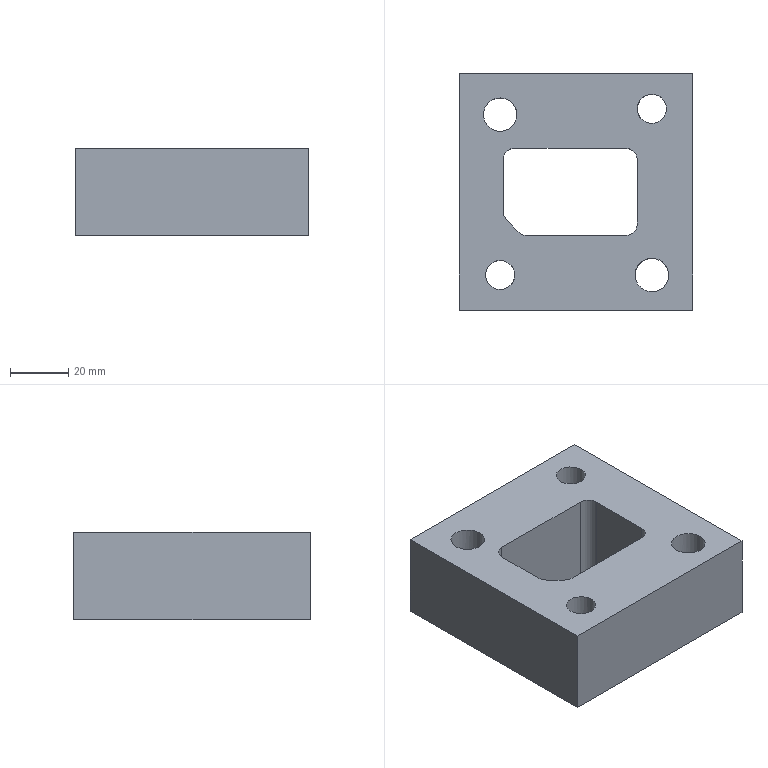Part | NX | features 7 2 | 1 solid | 28 faces | box 80 x 81 x 30 mm | volume 139031 mm3 | plane 15 | cylinder 13 | commonest cylinder face diameters 8 x5 10.001 x2 10.31 x2 11.5 x2 18 x2
STEP:
#1=CARTESIAN_POINT('',(3363.438,56.938,91.));
#2=VERTEX_POINT('',#1);
#3=CARTESIAN_POINT('',(3401.438,56.938,91.));
#4=VERTEX_POINT('',#3);
#5=CARTESIAN_POINT('',(3374.438,56.938,91.));
#6=DIRECTION('',(1.,0.,0.));
#7=VECTOR('',#6,1000.);
#8=LINE('',#5,#7);
#9=EDGE_CURVE('',#2,#4,#8,.T.);
#10=ORIENTED_EDGE('',*,*,#9,.T.);
#11=CARTESIAN_POINT('',(3405.438,52.938,91.));
#12=VERTEX_POINT('',#11);
#13=CARTESIAN_POINT('',(3401.438,52.938,91.));
#14=DIRECTION('',(0.,0.,1.));
#15=DIRECTION('',(0.,1.,0.));
#16=AXIS2_PLACEMENT_3D('',#13,#14,#15);
#17=CIRCLE('',#16,4.);
#18=EDGE_CURVE('',#12,#4,#17,.T.);
#19=ORIENTED_EDGE('',*,*,#18,.F.);
#20=CARTESIAN_POINT('',(3405.438,30.938,91.));
#21=VERTEX_POINT('',#20);
#22=CARTESIAN_POINT('',(3405.438,41.938,91.));
#23=DIRECTION('',(0.,-1.,0.));
#24=VECTOR('',#23,1000.);
#25=LINE('',#22,#24);
#26=EDGE_CURVE('',#12,#21,#25,.T.);
#27=ORIENTED_EDGE('',*,*,#26,.T.);
#28=CARTESIAN_POINT('',(3401.438,26.938,91.));
#29=VERTEX_POINT('',#28);
#30=CARTESIAN_POINT('',(3401.438,30.938,91.));
#31=DIRECTION('',(0.,0.,1.));
#32=DIRECTION('',(0.,1.,0.));
#33=AXIS2_PLACEMENT_3D('',#30,#31,#32);
#34=CIRCLE('',#33,4.);
#35=EDGE_CURVE('',#29,#21,#34,.T.);
#36=ORIENTED_EDGE('',*,*,#35,.F.);
#37=CARTESIAN_POINT('',(3367.731,26.938,91.));
#38=VERTEX_POINT('',#37);
#39=CARTESIAN_POINT('',(3374.438,26.938,91.));
#40=DIRECTION('',(-1.,0.,0.));
#41=VECTOR('',#40,1000.);
#42=LINE('',#39,#41);
#43=EDGE_CURVE('',#29,#38,#42,.T.);
#44=ORIENTED_EDGE('',*,*,#43,.T.);
#45=CARTESIAN_POINT('',(3364.902,28.11,91.));
#46=VERTEX_POINT('',#45);
#47=CARTESIAN_POINT('',(3367.731,30.938,91.));
#48=DIRECTION('',(0.,0.,1.));
#49=DIRECTION('',(0.,-1.,0.));
#50=AXIS2_PLACEMENT_3D('',#47,#48,#49);
#51=CIRCLE('',#50,4.);
#52=EDGE_CURVE('',#46,#38,#51,.T.);
#53=ORIENTED_EDGE('',*,*,#52,.F.);
#54=CARTESIAN_POINT('',(3360.609,32.403,91.));
#55=VERTEX_POINT('',#54);
#56=CARTESIAN_POINT('',(3364.006,29.006,91.));
#57=DIRECTION('',(0.7071,-0.7071,0.));
#58=VECTOR('',#57,1000.);
#59=LINE('',#56,#58);
#60=EDGE_CURVE('',#55,#46,#59,.T.);
#61=ORIENTED_EDGE('',*,*,#60,.F.);
#62=CARTESIAN_POINT('',(3359.438,35.231,91.));
#63=VERTEX_POINT('',#62);
#64=CARTESIAN_POINT('',(3363.438,35.231,91.));
#65=DIRECTION('',(0.,0.,1.));
#66=DIRECTION('',(0.,-1.,0.));
#67=AXIS2_PLACEMENT_3D('',#64,#65,#66);
#68=CIRCLE('',#67,4.);
#69=EDGE_CURVE('',#63,#55,#68,.T.);
#70=ORIENTED_EDGE('',*,*,#69,.F.);
#71=CARTESIAN_POINT('',(3359.438,52.938,91.));
#72=VERTEX_POINT('',#71);
#73=CARTESIAN_POINT('',(3359.438,41.938,91.));
#74=DIRECTION('',(0.,1.,0.));
#75=VECTOR('',#74,1000.);
#76=LINE('',#73,#75);
#77=EDGE_CURVE('',#63,#72,#76,.T.);
#78=ORIENTED_EDGE('',*,*,#77,.T.);
#79=CARTESIAN_POINT('',(3363.438,52.938,91.));
#80=DIRECTION('',(0.,0.,1.));
#81=DIRECTION('',(0.,-1.,0.));
#82=AXIS2_PLACEMENT_3D('',#79,#80,#81);
#83=CIRCLE('',#82,4.);
#84=EDGE_CURVE('',#2,#72,#83,.T.);
#85=ORIENTED_EDGE('',*,*,#84,.F.);
#86=EDGE_LOOP('',(#10,#19,#27,#36,#44,#53,#61,#70,#78,#85));
#87=FACE_BOUND('',#86,.T.);
#88=CARTESIAN_POINT('',(3410.438,75.439,91.));
#89=VERTEX_POINT('',#88);
#90=CARTESIAN_POINT('',(3410.438,70.438,91.));
#91=DIRECTION('',(0.,0.,-1.));
#92=DIRECTION('',(0.,1.,0.));
#93=AXIS2_PLACEMENT_3D('',#90,#91,#92);
#94=CIRCLE('',#93,5.);
#95=EDGE_CURVE('',#89,#89,#94,.T.);
#96=ORIENTED_EDGE('',*,*,#95,.T.);
#97=EDGE_LOOP('',(#96));
#98=FACE_BOUND('',#97,.T.);
#99=CARTESIAN_POINT('',(3358.438,74.188,91.));
#100=VERTEX_POINT('',#99);
#101=CARTESIAN_POINT('',(3358.438,68.438,91.));
#102=DIRECTION('',(0.,0.,1.));
#103=DIRECTION('',(0.,1.,0.));
#104=AXIS2_PLACEMENT_3D('',#101,#102,#103);
#105=CIRCLE('',#104,5.75);
#106=EDGE_CURVE('',#100,#100,#105,.T.);
#107=ORIENTED_EDGE('',*,*,#106,.F.);
#108=EDGE_LOOP('',(#107));
#109=FACE_BOUND('',#108,.T.);
#110=CARTESIAN_POINT('',(3424.438,1.438,91.));
#111=VERTEX_POINT('',#110);
#112=CARTESIAN_POINT('',(3344.438,1.438,91.));
#113=VERTEX_POINT('',#112);
#114=CARTESIAN_POINT('',(3374.438,1.438,91.));
#115=DIRECTION('',(-1.,0.,0.));
#116=VECTOR('',#115,1000.);
#117=LINE('',#114,#116);
#118=EDGE_CURVE('',#111,#113,#117,.T.);
#119=ORIENTED_EDGE('',*,*,#118,.F.);
#120=CARTESIAN_POINT('',(3424.438,82.438,91.));
#121=VERTEX_POINT('',#120);
#122=CARTESIAN_POINT('',(3424.438,41.938,91.));
#123=DIRECTION('',(0.,-1.,0.));
#124=VECTOR('',#123,1000.);
#125=LINE('',#122,#124);
#126=EDGE_CURVE('',#121,#111,#125,.T.);
#127=ORIENTED_EDGE('',*,*,#126,.F.);
#128=CARTESIAN_POINT('',(3344.438,82.438,91.));
#129=VERTEX_POINT('',#128);
#130=CARTESIAN_POINT('',(3374.438,82.438,91.));
#131=DIRECTION('',(1.,0.,0.));
#132=VECTOR('',#131,1000.);
#133=LINE('',#130,#132);
#134=EDGE_CURVE('',#129,#121,#133,.T.);
#135=ORIENTED_EDGE('',*,*,#134,.F.);
#136=CARTESIAN_POINT('',(3344.438,41.938,91.));
#137=DIRECTION('',(0.,1.,0.));
#138=VECTOR('',#137,1000.);
#139=LINE('',#136,#138);
#140=EDGE_CURVE('',#113,#129,#139,.T.);
#141=ORIENTED_EDGE('',*,*,#140,.F.);
#142=EDGE_LOOP('',(#119,#127,#135,#141));
#143=FACE_BOUND('',#142,.T.);
#144=CARTESIAN_POINT('',(3410.438,19.188,91.));
#145=VERTEX_POINT('',#144);
#146=CARTESIAN_POINT('',(3410.438,13.438,91.));
#147=DIRECTION('',(0.,0.,1.));
#148=DIRECTION('',(0.,1.,0.));
#149=AXIS2_PLACEMENT_3D('',#146,#147,#148);
#150=CIRCLE('',#149,5.75);
#151=EDGE_CURVE('',#145,#145,#150,.T.);
#152=ORIENTED_EDGE('',*,*,#151,.F.);
#153=EDGE_LOOP('',(#152));
#154=FACE_BOUND('',#153,.T.);
#155=CARTESIAN_POINT('',(3358.438,18.439,91.));
#156=VERTEX_POINT('',#155);
#157=CARTESIAN_POINT('',(3358.438,13.438,91.));
#158=DIRECTION('',(0.,0.,-1.));
#159=DIRECTION('',(0.,1.,0.));
#160=AXIS2_PLACEMENT_3D('',#157,#158,#159);
#161=CIRCLE('',#160,5.);
#162=EDGE_CURVE('',#156,#156,#161,.T.);
#163=ORIENTED_EDGE('',*,*,#162,.T.);
#164=EDGE_LOOP('',(#163));
#165=FACE_BOUND('',#164,.T.);
#166=CARTESIAN_POINT('',(3374.438,41.938,91.));
#167=DIRECTION('',(0.,0.,1.));
#168=DIRECTION('',(0.,-1.,0.));
#169=AXIS2_PLACEMENT_3D('',#166,#167,#168);
#170=PLANE('',#169);
#171=ADVANCED_FACE('',(#87,#98,#109,#143,#154,#165),#170,.T.);
#172=CARTESIAN_POINT('',(3415.593,70.438,61.));
#173=VERTEX_POINT('',#172);
#174=CARTESIAN_POINT('',(3410.438,70.438,61.));
#175=DIRECTION('',(0.,0.,1.));
#176=DIRECTION('',(1.,0.,0.));
#177=AXIS2_PLACEMENT_3D('',#174,#175,#176);
#178=CIRCLE('',#177,5.155);
#179=EDGE_CURVE('',#173,#173,#178,.T.);
#180=ORIENTED_EDGE('',*,*,#179,.T.);
#181=EDGE_LOOP('',(#180));
#182=FACE_BOUND('',#181,.T.);
#183=CARTESIAN_POINT('',(3363.593,13.438,61.));
#184=VERTEX_POINT('',#183);
#185=CARTESIAN_POINT('',(3358.438,13.438,61.));
#186=DIRECTION('',(0.,0.,1.));
#187=DIRECTION('',(1.,0.,0.));
#188=AXIS2_PLACEMENT_3D('',#185,#186,#187);
#189=CIRCLE('',#188,5.155);
#190=EDGE_CURVE('',#184,#184,#189,.T.);
#191=ORIENTED_EDGE('',*,*,#190,.T.);
#192=EDGE_LOOP('',(#191));
#193=FACE_BOUND('',#192,.T.);
#194=CARTESIAN_POINT('',(3359.438,52.938,61.));
#195=VERTEX_POINT('',#194);
#196=CARTESIAN_POINT('',(3363.438,56.938,61.));
#197=VERTEX_POINT('',#196);
#198=CARTESIAN_POINT('',(3363.438,52.938,61.));
#199=DIRECTION('',(0.,0.,-1.));
#200=DIRECTION('',(-1.,0.,0.));
#201=AXIS2_PLACEMENT_3D('',#198,#199,#200);
#202=CIRCLE('',#201,4.);
#203=EDGE_CURVE('',#195,#197,#202,.T.);
#204=ORIENTED_EDGE('',*,*,#203,.F.);
#205=CARTESIAN_POINT('',(3359.438,35.231,61.));
#206=VERTEX_POINT('',#205);
#207=CARTESIAN_POINT('',(3359.438,-135.062,61.));
#208=DIRECTION('',(0.,-1.,0.));
#209=VECTOR('',#208,1000.);
#210=LINE('',#207,#209);
#211=EDGE_CURVE('',#195,#206,#210,.T.);
#212=ORIENTED_EDGE('',*,*,#211,.T.);
#213=CARTESIAN_POINT('',(3360.609,32.403,61.));
#214=VERTEX_POINT('',#213);
#215=CARTESIAN_POINT('',(3363.438,35.231,61.));
#216=DIRECTION('',(0.,0.,-1.));
#217=DIRECTION('',(-1.,0.,0.));
#218=AXIS2_PLACEMENT_3D('',#215,#216,#217);
#219=CIRCLE('',#218,4.);
#220=EDGE_CURVE('',#214,#206,#219,.T.);
#221=ORIENTED_EDGE('',*,*,#220,.F.);
#222=CARTESIAN_POINT('',(3364.902,28.11,61.));
#223=VERTEX_POINT('',#222);
#224=CARTESIAN_POINT('',(3449.756,-56.744,61.));
#225=DIRECTION('',(-0.7071,0.7071,0.));
#226=VECTOR('',#225,1000.);
#227=LINE('',#224,#226);
#228=EDGE_CURVE('',#223,#214,#227,.T.);
#229=ORIENTED_EDGE('',*,*,#228,.F.);
#230=CARTESIAN_POINT('',(3367.731,26.938,61.));
#231=VERTEX_POINT('',#230);
#232=CARTESIAN_POINT('',(3367.731,30.938,61.));
#233=DIRECTION('',(0.,0.,-1.));
#234=DIRECTION('',(-1.,0.,0.));
#235=AXIS2_PLACEMENT_3D('',#232,#233,#234);
#236=CIRCLE('',#235,4.);
#237=EDGE_CURVE('',#231,#223,#236,.T.);
#238=ORIENTED_EDGE('',*,*,#237,.F.);
#239=CARTESIAN_POINT('',(3401.438,26.938,61.));
#240=VERTEX_POINT('',#239);
#241=CARTESIAN_POINT('',(3371.438,26.938,61.));
#242=DIRECTION('',(1.,0.,0.));
#243=VECTOR('',#242,1000.);
#244=LINE('',#241,#243);
#245=EDGE_CURVE('',#231,#240,#244,.T.);
#246=ORIENTED_EDGE('',*,*,#245,.T.);
#247=CARTESIAN_POINT('',(3405.438,30.938,61.));
#248=VERTEX_POINT('',#247);
#249=CARTESIAN_POINT('',(3401.438,30.938,61.));
#250=DIRECTION('',(0.,0.,-1.));
#251=DIRECTION('',(-1.,0.,0.));
#252=AXIS2_PLACEMENT_3D('',#249,#250,#251);
#253=CIRCLE('',#252,4.);
#254=EDGE_CURVE('',#248,#240,#253,.T.);
#255=ORIENTED_EDGE('',*,*,#254,.F.);
#256=CARTESIAN_POINT('',(3405.438,52.938,61.));
#257=VERTEX_POINT('',#256);
#258=CARTESIAN_POINT('',(3405.438,-135.062,61.));
#259=DIRECTION('',(0.,1.,0.));
#260=VECTOR('',#259,1000.);
#261=LINE('',#258,#260);
#262=EDGE_CURVE('',#248,#257,#261,.T.);
#263=ORIENTED_EDGE('',*,*,#262,.T.);
#264=CARTESIAN_POINT('',(3401.438,56.938,61.));
#265=VERTEX_POINT('',#264);
#266=CARTESIAN_POINT('',(3401.438,52.938,61.));
#267=DIRECTION('',(0.,0.,-1.));
#268=DIRECTION('',(-1.,0.,0.));
#269=AXIS2_PLACEMENT_3D('',#266,#267,#268);
#270=CIRCLE('',#269,4.);
#271=EDGE_CURVE('',#265,#257,#270,.T.);
#272=ORIENTED_EDGE('',*,*,#271,.F.);
#273=CARTESIAN_POINT('',(3371.438,56.938,61.));
#274=DIRECTION('',(-1.,0.,0.));
#275=VECTOR('',#274,1000.);
#276=LINE('',#273,#275);
#277=EDGE_CURVE('',#265,#197,#276,.T.);
#278=ORIENTED_EDGE('',*,*,#277,.T.);
#279=EDGE_LOOP('',(#204,#212,#221,#229,#238,#246,#255,#263,#272,#278));
#280=FACE_BOUND('',#279,.T.);
#281=CARTESIAN_POINT('',(3344.438,82.438,61.));
#282=VERTEX_POINT('',#281);
#283=CARTESIAN_POINT('',(3344.438,1.438,61.));
#284=VERTEX_POINT('',#283);
#285=CARTESIAN_POINT('',(3344.438,-135.062,61.));
#286=DIRECTION('',(0.,-1.,0.));
#287=VECTOR('',#286,1000.);
#288=LINE('',#285,#287);
#289=EDGE_CURVE('',#282,#284,#288,.T.);
#290=ORIENTED_EDGE('',*,*,#289,.F.);
#291=CARTESIAN_POINT('',(3424.438,82.438,61.));
#292=VERTEX_POINT('',#291);
#293=CARTESIAN_POINT('',(3371.438,82.438,61.));
#294=DIRECTION('',(-1.,0.,0.));
#295=VECTOR('',#294,1000.);
#296=LINE('',#293,#295);
#297=EDGE_CURVE('',#292,#282,#296,.T.);
#298=ORIENTED_EDGE('',*,*,#297,.F.);
#299=CARTESIAN_POINT('',(3424.438,1.438,61.));
#300=VERTEX_POINT('',#299);
#301=CARTESIAN_POINT('',(3424.438,-135.062,61.));
#302=DIRECTION('',(0.,1.,0.));
#303=VECTOR('',#302,1000.);
#304=LINE('',#301,#303);
#305=EDGE_CURVE('',#300,#292,#304,.T.);
#306=ORIENTED_EDGE('',*,*,#305,.F.);
#307=CARTESIAN_POINT('',(3371.438,1.438,61.));
#308=DIRECTION('',(1.,0.,0.));
#309=VECTOR('',#308,1000.);
#310=LINE('',#307,#309);
#311=EDGE_CURVE('',#284,#300,#310,.T.);
#312=ORIENTED_EDGE('',*,*,#311,.F.);
#313=EDGE_LOOP('',(#290,#298,#306,#312));
#314=FACE_BOUND('',#313,.T.);
#315=CARTESIAN_POINT('',(3401.438,13.438,61.));
#316=VERTEX_POINT('',#315);
#317=CARTESIAN_POINT('',(3410.438,13.438,61.));
#318=DIRECTION('',(0.,0.,1.));
#319=DIRECTION('',(-1.,0.,0.));
#320=AXIS2_PLACEMENT_3D('',#317,#318,#319);
#321=CIRCLE('',#320,9.);
#322=EDGE_CURVE('',#316,#316,#321,.T.);
#323=ORIENTED_EDGE('',*,*,#322,.T.);
#324=EDGE_LOOP('',(#323));
#325=FACE_BOUND('',#324,.T.);
#326=CARTESIAN_POINT('',(3349.438,68.438,61.));
#327=VERTEX_POINT('',#326);
#328=CARTESIAN_POINT('',(3358.438,68.438,61.));
#329=DIRECTION('',(0.,0.,1.));
#330=DIRECTION('',(-1.,0.,0.));
#331=AXIS2_PLACEMENT_3D('',#328,#329,#330);
#332=CIRCLE('',#331,9.);
#333=EDGE_CURVE('',#327,#327,#332,.T.);
#334=ORIENTED_EDGE('',*,*,#333,.T.);
#335=EDGE_LOOP('',(#334));
#336=FACE_BOUND('',#335,.T.);
#337=CARTESIAN_POINT('',(3371.438,-135.062,61.));
#338=DIRECTION('',(0.,0.,-1.));
#339=DIRECTION('',(0.,1.,0.));
#340=AXIS2_PLACEMENT_3D('',#337,#338,#339);
#341=PLANE('',#340);
#342=ADVANCED_FACE('',(#182,#193,#280,#314,#325,#336),#341,.T.);
#343=ORIENTED_EDGE('',*,*,#140,.T.);
#344=CARTESIAN_POINT('',(3344.438,82.438,6.933));
#345=DIRECTION('',(0.,0.,-1.));
#346=VECTOR('',#345,1000.);
#347=LINE('',#344,#346);
#348=EDGE_CURVE('',#129,#282,#347,.T.);
#349=ORIENTED_EDGE('',*,*,#348,.T.);
#350=ORIENTED_EDGE('',*,*,#289,.T.);
#351=CARTESIAN_POINT('',(3344.438,1.438,6.933));
#352=DIRECTION('',(0.,0.,-1.));
#353=VECTOR('',#352,1000.);
#354=LINE('',#351,#353);
#355=EDGE_CURVE('',#113,#284,#354,.T.);
#356=ORIENTED_EDGE('',*,*,#355,.F.);
#357=EDGE_LOOP('',(#343,#349,#350,#356));
#358=FACE_BOUND('',#357,.T.);
#359=CARTESIAN_POINT('',(3344.438,41.938,6.933));
#360=DIRECTION('',(-1.,0.,0.));
#361=DIRECTION('',(0.,0.,-1.));
#362=AXIS2_PLACEMENT_3D('',#359,#360,#361);
#363=PLANE('',#362);
#364=ADVANCED_FACE('',(#358),#363,.T.);
#365=ORIENTED_EDGE('',*,*,#134,.T.);
#366=CARTESIAN_POINT('',(3424.438,82.438,6.933));
#367=DIRECTION('',(0.,0.,-1.));
#368=VECTOR('',#367,1000.);
#369=LINE('',#366,#368);
#370=EDGE_CURVE('',#121,#292,#369,.T.);
#371=ORIENTED_EDGE('',*,*,#370,.T.);
#372=ORIENTED_EDGE('',*,*,#297,.T.);
#373=ORIENTED_EDGE('',*,*,#348,.F.);
#374=EDGE_LOOP('',(#365,#371,#372,#373));
#375=FACE_BOUND('',#374,.T.);
#376=CARTESIAN_POINT('',(3374.438,82.438,6.933));
#377=DIRECTION('',(0.,1.,0.));
#378=DIRECTION('',(0.,0.,1.));
#379=AXIS2_PLACEMENT_3D('',#376,#377,#378);
#380=PLANE('',#379);
#381=ADVANCED_FACE('',(#375),#380,.T.);
#382=ORIENTED_EDGE('',*,*,#126,.T.);
#383=CARTESIAN_POINT('',(3424.438,1.438,6.933));
#384=DIRECTION('',(0.,0.,1.));
#385=VECTOR('',#384,1000.);
#386=LINE('',#383,#385);
#387=EDGE_CURVE('',#300,#111,#386,.T.);
#388=ORIENTED_EDGE('',*,*,#387,.F.);
#389=ORIENTED_EDGE('',*,*,#305,.T.);
#390=ORIENTED_EDGE('',*,*,#370,.F.);
#391=EDGE_LOOP('',(#382,#388,#389,#390));
#392=FACE_BOUND('',#391,.T.);
#393=CARTESIAN_POINT('',(3424.438,41.938,6.933));
#394=DIRECTION('',(1.,0.,0.));
#395=DIRECTION('',(0.,0.,1.));
#396=AXIS2_PLACEMENT_3D('',#393,#394,#395);
#397=PLANE('',#396);
#398=ADVANCED_FACE('',(#392),#397,.T.);
#399=ORIENTED_EDGE('',*,*,#311,.T.);
#400=ORIENTED_EDGE('',*,*,#387,.T.);
#401=ORIENTED_EDGE('',*,*,#118,.T.);
#402=ORIENTED_EDGE('',*,*,#355,.T.);
#403=EDGE_LOOP('',(#399,#400,#401,#402));
#404=FACE_BOUND('',#403,.T.);
#405=CARTESIAN_POINT('',(3374.438,1.438,6.933));
#406=DIRECTION('',(0.,-1.,0.));
#407=DIRECTION('',(0.,0.,-1.));
#408=AXIS2_PLACEMENT_3D('',#405,#406,#407);
#409=PLANE('',#408);
#410=ADVANCED_FACE('',(#404),#409,.T.);
#411=ORIENTED_EDGE('',*,*,#151,.T.);
#412=EDGE_LOOP('',(#411));
#413=FACE_BOUND('',#412,.T.);
#414=CARTESIAN_POINT('',(3416.188,13.438,74.));
#415=VERTEX_POINT('',#414);
#416=CARTESIAN_POINT('',(3410.438,13.438,74.));
#417=DIRECTION('',(0.,0.,1.));
#418=DIRECTION('',(1.,0.,0.));
#419=AXIS2_PLACEMENT_3D('',#416,#417,#418);
#420=CIRCLE('',#419,5.75);
#421=EDGE_CURVE('',#415,#415,#420,.T.);
#422=ORIENTED_EDGE('',*,*,#421,.F.);
#423=EDGE_LOOP('',(#422));
#424=FACE_BOUND('',#423,.T.);
#425=CARTESIAN_POINT('',(3410.438,13.438,51.));
#426=DIRECTION('',(0.,0.,1.));
#427=DIRECTION('',(0.,-1.,0.));
#428=AXIS2_PLACEMENT_3D('',#425,#426,#427);
#429=CYLINDRICAL_SURFACE('',#428,5.75);
#430=ADVANCED_FACE('',(#413,#424),#429,.F.);
#431=ORIENTED_EDGE('',*,*,#421,.T.);
#432=EDGE_LOOP('',(#431));
#433=FACE_BOUND('',#432,.T.);
#434=CARTESIAN_POINT('',(3419.438,13.438,74.));
#435=VERTEX_POINT('',#434);
#436=CARTESIAN_POINT('',(3410.438,13.438,74.));
#437=DIRECTION('',(0.,0.,1.));
#438=DIRECTION('',(1.,0.,0.));
#439=AXIS2_PLACEMENT_3D('',#436,#437,#438);
#440=CIRCLE('',#439,9.);
#441=EDGE_CURVE('',#435,#435,#440,.T.);
#442=ORIENTED_EDGE('',*,*,#441,.F.);
#443=EDGE_LOOP('',(#442));
#444=FACE_BOUND('',#443,.T.);
#445=CARTESIAN_POINT('',(3222.438,13.438,74.));
#446=DIRECTION('',(0.,0.,1.));
#447=DIRECTION('',(0.,-1.,0.));
#448=AXIS2_PLACEMENT_3D('',#445,#446,#447);
#449=PLANE('',#448);
#450=ADVANCED_FACE('',(#433,#444),#449,.F.);
#451=ORIENTED_EDGE('',*,*,#441,.T.);
#452=EDGE_LOOP('',(#451));
#453=FACE_BOUND('',#452,.T.);
#454=ORIENTED_EDGE('',*,*,#322,.F.);
#455=EDGE_LOOP('',(#454));
#456=FACE_BOUND('',#455,.T.);
#457=CARTESIAN_POINT('',(3410.438,13.438,56.));
#458=DIRECTION('',(0.,0.,1.));
#459=DIRECTION('',(0.,-1.,0.));
#460=AXIS2_PLACEMENT_3D('',#457,#458,#459);
#461=CYLINDRICAL_SURFACE('',#460,9.);
#462=ADVANCED_FACE('',(#453,#456),#461,.F.);
#463=CARTESIAN_POINT('',(3363.438,13.438,71.));
#464=VERTEX_POINT('',#463);
#465=CARTESIAN_POINT('',(3358.438,13.438,71.));
#466=DIRECTION('',(0.,0.,-1.));
#467=DIRECTION('',(1.,0.,0.));
#468=AXIS2_PLACEMENT_3D('',#465,#466,#467);
#469=CIRCLE('',#468,5.);
#470=EDGE_CURVE('',#464,#464,#469,.T.);
#471=ORIENTED_EDGE('',*,*,#470,.T.);
#472=EDGE_LOOP('',(#471));
#473=FACE_BOUND('',#472,.T.);
#474=ORIENTED_EDGE('',*,*,#162,.F.);
#475=EDGE_LOOP('',(#474));
#476=FACE_BOUND('',#475,.T.);
#477=CARTESIAN_POINT('',(3358.438,13.438,621.));
#478=DIRECTION('',(0.,0.,-1.));
#479=DIRECTION('',(0.,1.,0.));
#480=AXIS2_PLACEMENT_3D('',#477,#478,#479);
#481=CYLINDRICAL_SURFACE('',#480,5.);
#482=ADVANCED_FACE('',(#473,#476),#481,.F.);
#483=ORIENTED_EDGE('',*,*,#106,.T.);
#484=EDGE_LOOP('',(#483));
#485=FACE_BOUND('',#484,.T.);
#486=CARTESIAN_POINT('',(3364.188,68.438,74.));
#487=VERTEX_POINT('',#486);
#488=CARTESIAN_POINT('',(3358.438,68.438,74.));
#489=DIRECTION('',(0.,0.,1.));
#490=DIRECTION('',(1.,0.,0.));
#491=AXIS2_PLACEMENT_3D('',#488,#489,#490);
#492=CIRCLE('',#491,5.75);
#493=EDGE_CURVE('',#487,#487,#492,.T.);
#494=ORIENTED_EDGE('',*,*,#493,.F.);
#495=EDGE_LOOP('',(#494));
#496=FACE_BOUND('',#495,.T.);
#497=CARTESIAN_POINT('',(3358.438,68.438,51.));
#498=DIRECTION('',(0.,0.,1.));
#499=DIRECTION('',(0.,-1.,0.));
#500=AXIS2_PLACEMENT_3D('',#497,#498,#499);
#501=CYLINDRICAL_SURFACE('',#500,5.75);
#502=ADVANCED_FACE('',(#485,#496),#501,.F.);
#503=ORIENTED_EDGE('',*,*,#493,.T.);
#504=EDGE_LOOP('',(#503));
#505=FACE_BOUND('',#504,.T.);
#506=CARTESIAN_POINT('',(3367.438,68.438,74.));
#507=VERTEX_POINT('',#506);
#508=CARTESIAN_POINT('',(3358.438,68.438,74.));
#509=DIRECTION('',(0.,0.,1.));
#510=DIRECTION('',(1.,0.,0.));
#511=AXIS2_PLACEMENT_3D('',#508,#509,#510);
#512=CIRCLE('',#511,9.);
#513=EDGE_CURVE('',#507,#507,#512,.T.);
#514=ORIENTED_EDGE('',*,*,#513,.F.);
#515=EDGE_LOOP('',(#514));
#516=FACE_BOUND('',#515,.T.);
#517=CARTESIAN_POINT('',(3222.438,13.438,74.));
#518=DIRECTION('',(0.,0.,1.));
#519=DIRECTION('',(0.,-1.,0.));
#520=AXIS2_PLACEMENT_3D('',#517,#518,#519);
#521=PLANE('',#520);
#522=ADVANCED_FACE('',(#505,#516),#521,.F.);
#523=ORIENTED_EDGE('',*,*,#513,.T.);
#524=EDGE_LOOP('',(#523));
#525=FACE_BOUND('',#524,.T.);
#526=ORIENTED_EDGE('',*,*,#333,.F.);
#527=EDGE_LOOP('',(#526));
#528=FACE_BOUND('',#527,.T.);
#529=CARTESIAN_POINT('',(3358.438,68.438,56.));
#530=DIRECTION('',(0.,0.,1.));
#531=DIRECTION('',(0.,-1.,0.));
#532=AXIS2_PLACEMENT_3D('',#529,#530,#531);
#533=CYLINDRICAL_SURFACE('',#532,9.);
#534=ADVANCED_FACE('',(#525,#528),#533,.F.);
#535=CARTESIAN_POINT('',(3415.438,70.438,71.));
#536=VERTEX_POINT('',#535);
#537=CARTESIAN_POINT('',(3410.438,70.438,71.));
#538=DIRECTION('',(0.,0.,-1.));
#539=DIRECTION('',(1.,0.,0.));
#540=AXIS2_PLACEMENT_3D('',#537,#538,#539);
#541=CIRCLE('',#540,5.);
#542=EDGE_CURVE('',#536,#536,#541,.T.);
#543=ORIENTED_EDGE('',*,*,#542,.T.);
#544=EDGE_LOOP('',(#543));
#545=FACE_BOUND('',#544,.T.);
#546=ORIENTED_EDGE('',*,*,#95,.F.);
#547=EDGE_LOOP('',(#546));
#548=FACE_BOUND('',#547,.T.);
#549=CARTESIAN_POINT('',(3410.438,70.438,621.));
#550=DIRECTION('',(0.,0.,-1.));
#551=DIRECTION('',(0.,1.,0.));
#552=AXIS2_PLACEMENT_3D('',#549,#550,#551);
#553=CYLINDRICAL_SURFACE('',#552,5.);
#554=ADVANCED_FACE('',(#545,#548),#553,.F.);
#555=ORIENTED_EDGE('',*,*,#9,.F.);
#556=CARTESIAN_POINT('',(3363.438,56.938,-5.));
#557=DIRECTION('',(0.,0.,1.));
#558=VECTOR('',#557,1000.);
#559=LINE('',#556,#558);
#560=EDGE_CURVE('',#197,#2,#559,.T.);
#561=ORIENTED_EDGE('',*,*,#560,.F.);
#562=ORIENTED_EDGE('',*,*,#277,.F.);
#563=CARTESIAN_POINT('',(3401.438,56.938,-5.));
#564=DIRECTION('',(0.,0.,1.));
#565=VECTOR('',#564,1000.);
#566=LINE('',#563,#565);
#567=EDGE_CURVE('',#265,#4,#566,.T.);
#568=ORIENTED_EDGE('',*,*,#567,.T.);
#569=EDGE_LOOP('',(#555,#561,#562,#568));
#570=FACE_BOUND('',#569,.T.);
#571=CARTESIAN_POINT('',(3374.438,56.938,-5.));
#572=DIRECTION('',(0.,1.,0.));
#573=DIRECTION('',(0.,0.,1.));
#574=AXIS2_PLACEMENT_3D('',#571,#572,#573);
#575=PLANE('',#574);
#576=ADVANCED_FACE('',(#570),#575,.F.);
#577=ORIENTED_EDGE('',*,*,#26,.F.);
#578=CARTESIAN_POINT('',(3405.438,52.938,-5.));
#579=DIRECTION('',(0.,0.,-1.));
#580=VECTOR('',#579,1000.);
#581=LINE('',#578,#580);
#582=EDGE_CURVE('',#12,#257,#581,.T.);
#583=ORIENTED_EDGE('',*,*,#582,.T.);
#584=ORIENTED_EDGE('',*,*,#262,.F.);
#585=CARTESIAN_POINT('',(3405.438,30.938,-5.));
#586=DIRECTION('',(0.,0.,1.));
#587=VECTOR('',#586,1000.);
#588=LINE('',#585,#587);
#589=EDGE_CURVE('',#248,#21,#588,.T.);
#590=ORIENTED_EDGE('',*,*,#589,.T.);
#591=EDGE_LOOP('',(#577,#583,#584,#590));
#592=FACE_BOUND('',#591,.T.);
#593=CARTESIAN_POINT('',(3405.438,41.938,-5.));
#594=DIRECTION('',(1.,0.,0.));
#595=DIRECTION('',(0.,0.,1.));
#596=AXIS2_PLACEMENT_3D('',#593,#594,#595);
#597=PLANE('',#596);
#598=ADVANCED_FACE('',(#592),#597,.F.);
#599=ORIENTED_EDGE('',*,*,#245,.F.);
#600=CARTESIAN_POINT('',(3367.731,26.938,-5.));
#601=DIRECTION('',(0.,0.,-1.));
#602=VECTOR('',#601,1000.);
#603=LINE('',#600,#602);
#604=EDGE_CURVE('',#38,#231,#603,.T.);
#605=ORIENTED_EDGE('',*,*,#604,.F.);
#606=ORIENTED_EDGE('',*,*,#43,.F.);
#607=CARTESIAN_POINT('',(3401.438,26.938,-5.));
#608=DIRECTION('',(0.,0.,-1.));
#609=VECTOR('',#608,1000.);
#610=LINE('',#607,#609);
#611=EDGE_CURVE('',#29,#240,#610,.T.);
#612=ORIENTED_EDGE('',*,*,#611,.T.);
#613=EDGE_LOOP('',(#599,#605,#606,#612));
#614=FACE_BOUND('',#613,.T.);
#615=CARTESIAN_POINT('',(3374.438,26.938,-5.));
#616=DIRECTION('',(0.,-1.,0.));
#617=DIRECTION('',(0.,0.,-1.));
#618=AXIS2_PLACEMENT_3D('',#615,#616,#617);
#619=PLANE('',#618);
#620=ADVANCED_FACE('',(#614),#619,.F.);
#621=ORIENTED_EDGE('',*,*,#254,.T.);
#622=ORIENTED_EDGE('',*,*,#611,.F.);
#623=ORIENTED_EDGE('',*,*,#35,.T.);
#624=ORIENTED_EDGE('',*,*,#589,.F.);
#625=EDGE_LOOP('',(#621,#622,#623,#624));
#626=FACE_BOUND('',#625,.T.);
#627=CARTESIAN_POINT('',(3401.438,30.938,-5.));
#628=DIRECTION('',(0.,0.,-1.));
#629=DIRECTION('',(0.,-1.,0.));
#630=AXIS2_PLACEMENT_3D('',#627,#628,#629);
#631=CYLINDRICAL_SURFACE('',#630,4.);
#632=ADVANCED_FACE('',(#626),#631,.F.);
#633=ORIENTED_EDGE('',*,*,#271,.T.);
#634=ORIENTED_EDGE('',*,*,#582,.F.);
#635=ORIENTED_EDGE('',*,*,#18,.T.);
#636=ORIENTED_EDGE('',*,*,#567,.F.);
#637=EDGE_LOOP('',(#633,#634,#635,#636));
#638=FACE_BOUND('',#637,.T.);
#639=CARTESIAN_POINT('',(3401.438,52.938,-5.));
#640=DIRECTION('',(0.,0.,-1.));
#641=DIRECTION('',(0.,-1.,0.));
#642=AXIS2_PLACEMENT_3D('',#639,#640,#641);
#643=CYLINDRICAL_SURFACE('',#642,4.);
#644=ADVANCED_FACE('',(#638),#643,.F.);
#645=ORIENTED_EDGE('',*,*,#77,.F.);
#646=CARTESIAN_POINT('',(3359.438,35.231,-5.));
#647=DIRECTION('',(0.,0.,-1.));
#648=VECTOR('',#647,1000.);
#649=LINE('',#646,#648);
#650=EDGE_CURVE('',#63,#206,#649,.T.);
#651=ORIENTED_EDGE('',*,*,#650,.T.);
#652=ORIENTED_EDGE('',*,*,#211,.F.);
#653=CARTESIAN_POINT('',(3359.438,52.938,-5.));
#654=DIRECTION('',(0.,0.,1.));
#655=VECTOR('',#654,1000.);
#656=LINE('',#653,#655);
#657=EDGE_CURVE('',#195,#72,#656,.T.);
#658=ORIENTED_EDGE('',*,*,#657,.T.);
#659=EDGE_LOOP('',(#645,#651,#652,#658));
#660=FACE_BOUND('',#659,.T.);
#661=CARTESIAN_POINT('',(3359.438,41.938,-5.));
#662=DIRECTION('',(-1.,0.,0.));
#663=DIRECTION('',(0.,0.,-1.));
#664=AXIS2_PLACEMENT_3D('',#661,#662,#663);
#665=PLANE('',#664);
#666=ADVANCED_FACE('',(#660),#665,.F.);
#667=ORIENTED_EDGE('',*,*,#60,.T.);
#668=CARTESIAN_POINT('',(3364.902,28.11,-5.));
#669=DIRECTION('',(0.,0.,-1.));
#670=VECTOR('',#669,1000.);
#671=LINE('',#668,#670);
#672=EDGE_CURVE('',#46,#223,#671,.T.);
#673=ORIENTED_EDGE('',*,*,#672,.T.);
#674=ORIENTED_EDGE('',*,*,#228,.T.);
#675=CARTESIAN_POINT('',(3360.609,32.403,-5.));
#676=DIRECTION('',(0.,0.,1.));
#677=VECTOR('',#676,1000.);
#678=LINE('',#675,#677);
#679=EDGE_CURVE('',#214,#55,#678,.T.);
#680=ORIENTED_EDGE('',*,*,#679,.T.);
#681=EDGE_LOOP('',(#667,#673,#674,#680));
#682=FACE_BOUND('',#681,.T.);
#683=CARTESIAN_POINT('',(3366.756,26.256,-5.));
#684=DIRECTION('',(0.7071,0.7071,0.));
#685=DIRECTION('',(0.,0.,1.));
#686=AXIS2_PLACEMENT_3D('',#683,#684,#685);
#687=PLANE('',#686);
#688=ADVANCED_FACE('',(#682),#687,.T.);
#689=ORIENTED_EDGE('',*,*,#237,.T.);
#690=ORIENTED_EDGE('',*,*,#672,.F.);
#691=ORIENTED_EDGE('',*,*,#52,.T.);
#692=ORIENTED_EDGE('',*,*,#604,.T.);
#693=EDGE_LOOP('',(#689,#690,#691,#692));
#694=FACE_BOUND('',#693,.T.);
#695=CARTESIAN_POINT('',(3367.731,30.938,-5.));
#696=DIRECTION('',(0.,0.,1.));
#697=DIRECTION('',(0.,-1.,0.));
#698=AXIS2_PLACEMENT_3D('',#695,#696,#697);
#699=CYLINDRICAL_SURFACE('',#698,4.);
#700=ADVANCED_FACE('',(#694),#699,.F.);
#701=ORIENTED_EDGE('',*,*,#69,.T.);
#702=ORIENTED_EDGE('',*,*,#679,.F.);
#703=ORIENTED_EDGE('',*,*,#220,.T.);
#704=ORIENTED_EDGE('',*,*,#650,.F.);
#705=EDGE_LOOP('',(#701,#702,#703,#704));
#706=FACE_BOUND('',#705,.T.);
#707=CARTESIAN_POINT('',(3363.438,35.231,-5.));
#708=DIRECTION('',(0.,0.,-1.));
#709=DIRECTION('',(0.,1.,0.));
#710=AXIS2_PLACEMENT_3D('',#707,#708,#709);
#711=CYLINDRICAL_SURFACE('',#710,4.);
#712=ADVANCED_FACE('',(#706),#711,.F.);
#713=ORIENTED_EDGE('',*,*,#203,.T.);
#714=ORIENTED_EDGE('',*,*,#560,.T.);
#715=ORIENTED_EDGE('',*,*,#84,.T.);
#716=ORIENTED_EDGE('',*,*,#657,.F.);
#717=EDGE_LOOP('',(#713,#714,#715,#716));
#718=FACE_BOUND('',#717,.T.);
#719=CARTESIAN_POINT('',(3363.438,52.938,-5.));
#720=DIRECTION('',(0.,0.,-1.));
#721=DIRECTION('',(0.,1.,0.));
#722=AXIS2_PLACEMENT_3D('',#719,#720,#721);
#723=CYLINDRICAL_SURFACE('',#722,4.);
#724=ADVANCED_FACE('',(#718),#723,.F.);
#725=CARTESIAN_POINT('',(3363.593,13.438,71.));
#726=VERTEX_POINT('',#725);
#727=CARTESIAN_POINT('',(3358.438,13.438,71.));
#728=DIRECTION('',(0.,0.,-1.));
#729=DIRECTION('',(1.,0.,0.));
#730=AXIS2_PLACEMENT_3D('',#727,#728,#729);
#731=CIRCLE('',#730,5.155);
#732=EDGE_CURVE('',#726,#726,#731,.T.);
#733=ORIENTED_EDGE('',*,*,#732,.T.);
#734=EDGE_LOOP('',(#733));
#735=FACE_BOUND('',#734,.T.);
#736=ORIENTED_EDGE('',*,*,#470,.F.);
#737=EDGE_LOOP('',(#736));
#738=FACE_BOUND('',#737,.T.);
#739=CARTESIAN_POINT('',(3358.438,13.438,71.));
#740=DIRECTION('',(0.,0.,1.));
#741=DIRECTION('',(-1.,0.,0.));
#742=AXIS2_PLACEMENT_3D('',#739,#740,#741);
#743=PLANE('',#742);
#744=ADVANCED_FACE('',(#735,#738),#743,.F.);
#745=ORIENTED_EDGE('',*,*,#732,.F.);
#746=EDGE_LOOP('',(#745));
#747=FACE_BOUND('',#746,.T.);
#748=ORIENTED_EDGE('',*,*,#190,.F.);
#749=EDGE_LOOP('',(#748));
#750=FACE_BOUND('',#749,.T.);
#751=CARTESIAN_POINT('',(3358.438,13.438,61.));
#752=DIRECTION('',(0.,0.,1.));
#753=DIRECTION('',(-1.,0.,0.));
#754=AXIS2_PLACEMENT_3D('',#751,#752,#753);
#755=CYLINDRICAL_SURFACE('',#754,5.155);
#756=ADVANCED_FACE('',(#747,#750),#755,.F.);
#757=CARTESIAN_POINT('',(3415.593,70.438,71.));
#758=VERTEX_POINT('',#757);
#759=CARTESIAN_POINT('',(3410.438,70.438,71.));
#760=DIRECTION('',(0.,0.,-1.));
#761=DIRECTION('',(1.,0.,0.));
#762=AXIS2_PLACEMENT_3D('',#759,#760,#761);
#763=CIRCLE('',#762,5.155);
#764=EDGE_CURVE('',#758,#758,#763,.T.);
#765=ORIENTED_EDGE('',*,*,#764,.T.);
#766=EDGE_LOOP('',(#765));
#767=FACE_BOUND('',#766,.T.);
#768=ORIENTED_EDGE('',*,*,#542,.F.);
#769=EDGE_LOOP('',(#768));
#770=FACE_BOUND('',#769,.T.);
#771=CARTESIAN_POINT('',(3410.438,70.438,71.));
#772=DIRECTION('',(0.,0.,1.));
#773=DIRECTION('',(-1.,0.,0.));
#774=AXIS2_PLACEMENT_3D('',#771,#772,#773);
#775=PLANE('',#774);
#776=ADVANCED_FACE('',(#767,#770),#775,.F.);
#777=ORIENTED_EDGE('',*,*,#764,.F.);
#778=EDGE_LOOP('',(#777));
#779=FACE_BOUND('',#778,.T.);
#780=ORIENTED_EDGE('',*,*,#179,.F.);
#781=EDGE_LOOP('',(#780));
#782=FACE_BOUND('',#781,.T.);
#783=CARTESIAN_POINT('',(3410.438,70.438,61.));
#784=DIRECTION('',(0.,0.,1.));
#785=DIRECTION('',(-1.,0.,0.));
#786=AXIS2_PLACEMENT_3D('',#783,#784,#785);
#787=CYLINDRICAL_SURFACE('',#786,5.155);
#788=ADVANCED_FACE('',(#779,#782),#787,.F.);
#789=CLOSED_SHELL('',(#171,#342,#364,#381,#398,#410,#430,#450,#462,#482,#502,#522,#534,#554,#576,#598,#620,#632,#644,#666,#688,#700,#712,#724,#744,#756,#776,#788));
#790=MANIFOLD_SOLID_BREP('',#789);
#791=(LENGTH_UNIT()NAMED_UNIT(*)SI_UNIT(.MILLI.,.METRE.));
#792=UNCERTAINTY_MEASURE_WITH_UNIT(LENGTH_MEASURE(0.00001),#791,'','');
#793=(NAMED_UNIT(*)PLANE_ANGLE_UNIT()SI_UNIT($,.RADIAN.));
#794=(NAMED_UNIT(*)SI_UNIT($,.STERADIAN.)SOLID_ANGLE_UNIT());
#795=(GEOMETRIC_REPRESENTATION_CONTEXT(3)GLOBAL_UNCERTAINTY_ASSIGNED_CONTEXT((#792))GLOBAL_UNIT_ASSIGNED_CONTEXT((#791,#793,#794))REPRESENTATION_CONTEXT('',''));
#796=ADVANCED_BREP_SHAPE_REPRESENTATION('',(#790),#795);